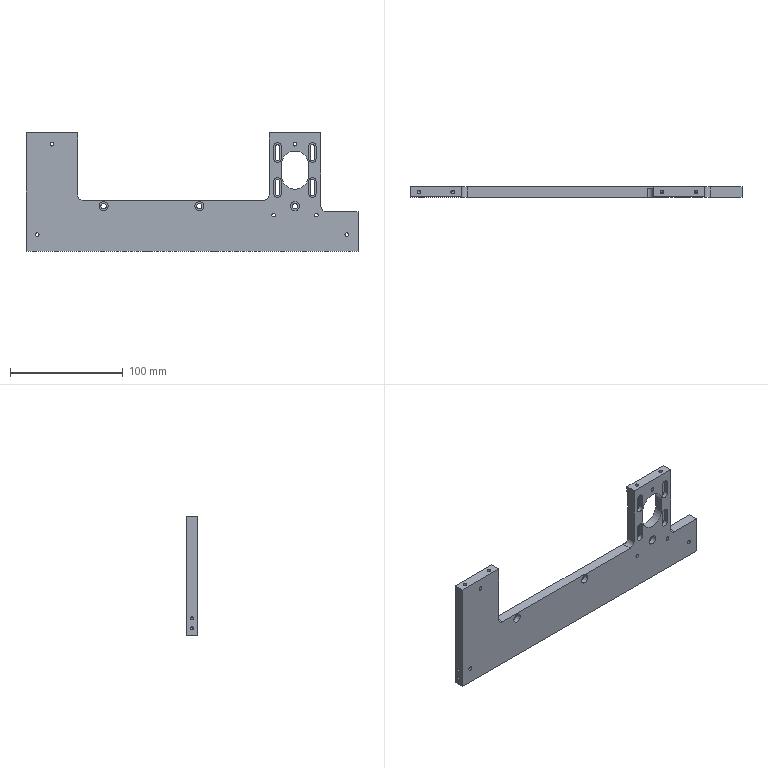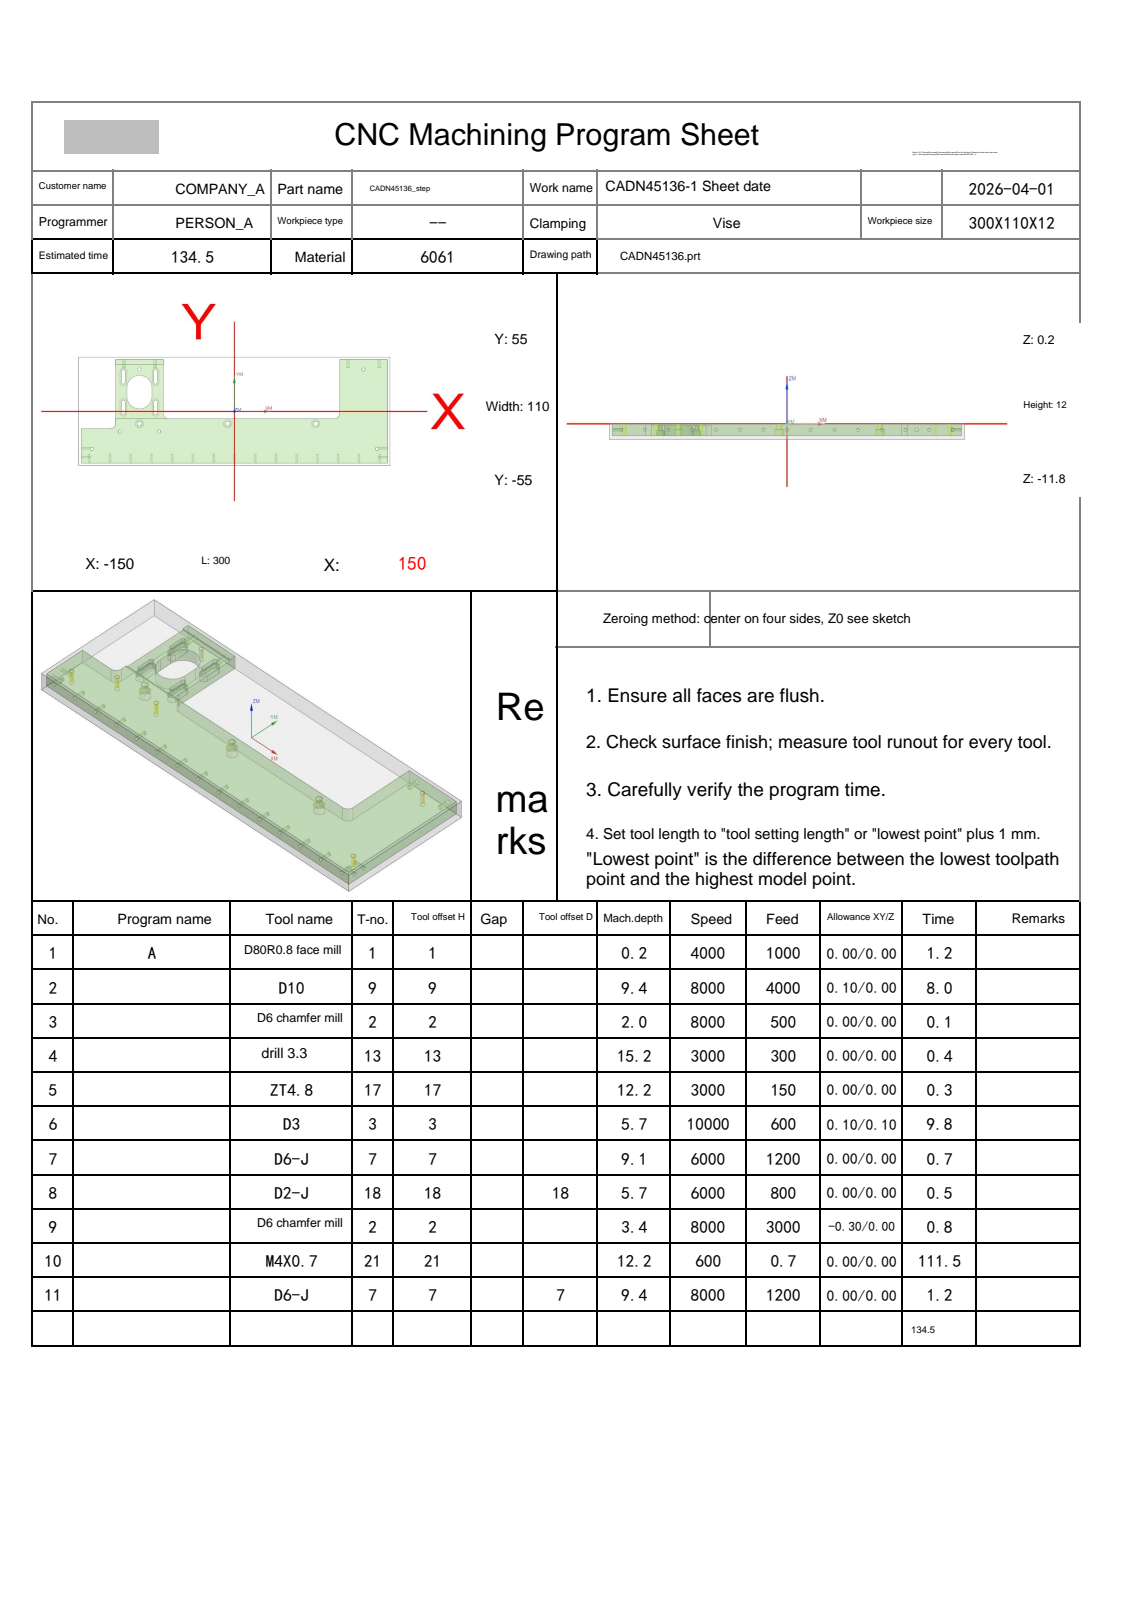NC program | NX | posted by the shop | part box 295 x 9 x 105 mm
Lines 3202 to 3255 of 7463:
N3 T02 M06
(D6 chamfer mill  D=6. R=0. H=02 ce=0.00 di=0.00)
G00 G90 G54 X-91.5 Y42.5 M03 S8000
G43 H02 Z20.
M08
G98 G81 X-91.5 Y42.5 Z-1.8 R0.0 F500.
X-137.5 Y-38. Z-.8 R1.
X-110.5 Y-20.5
X-91.5 Y-12.5
X-72.5 Y-20.5
X-6.5 Y-12.5
X78.5
X137.5 Y-38.
X124.5 Y42.5
G80
G00 Z20.
G91 G28 Z0.0
M05
M09
G91 G28 Z0.0
M01
N4 T13 M06
(drill 3.3 D=3.3 DR_a=118 H=13)
G00 G90 G54 X137.5 Y-38. M03 S3000
G43 H13 Z20.
M08
G98 G83 X137.5 Y-38. Z-14.991 R1. F300. Q2.
X124.5 Y42.5
G98 G83 X-91.5 Y42.5 Z-14.991 R0.0 Q2.
G98 G83 X-72.5 Y-20.5 Z-14.991 R1. Q2.
X-110.5
X-137.5 Y-38.
G80
G00 Z20.
G91 G28 Z0.0
M05
M09
G91 G28 Z0.0
M01
N5 T17 M06
(ZT4.8 D=4.8 DR_a=118 H=17)
G00 G90 G54 X78.5 Y-12.5 M03 S3000
G43 H17 Z20.
M08
G98 G83 X78.5 Y-12.5 Z-12. R1. F150. Q3.
X-6.5
X-91.5
G80
G00 Z20.
G91 G28 Z0.0
M05
M09
G91 G28 Z0.0
M01